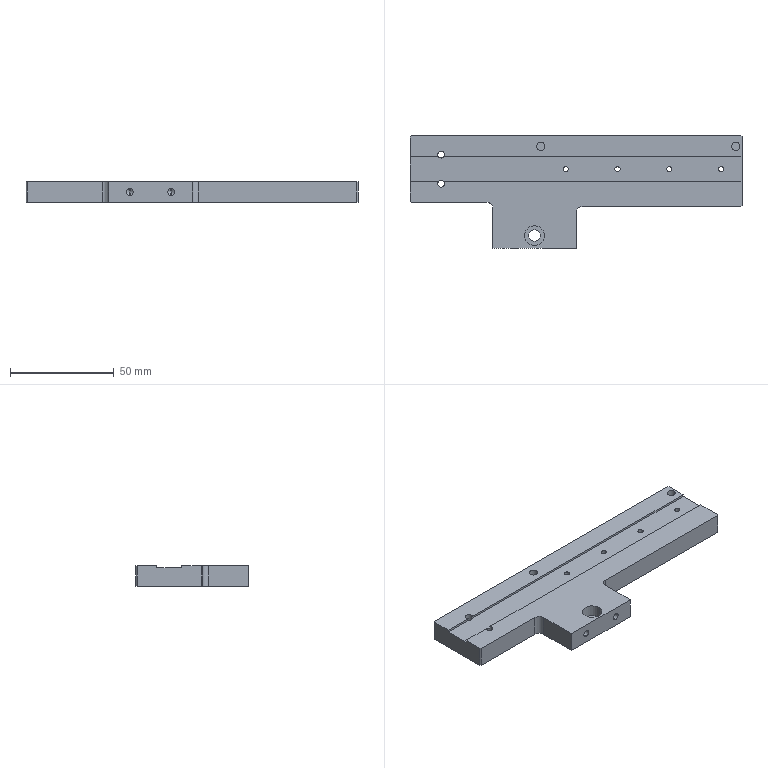Part | STEP file | PN_0013 Mount electronic clip mounting plate 1 | 1 solid | 53 faces | box 160 x 54 x 10 mm | volume 58459 mm3 | cylinder 26 | plane 23 | cone 4 | commonest cylinder face diameters 2.5 x8 3.3 x8 4 x4 5.5 x2 6 x2 9.5 x2